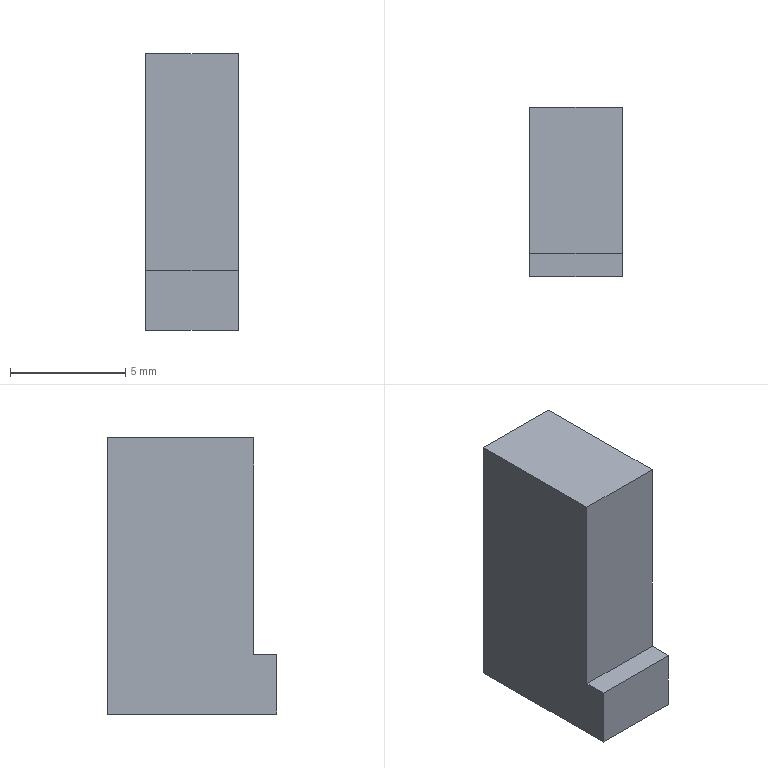Part | STEP file | lll_id462_x_t | 1 solid | 8 faces | box 4 x 7.35 x 12 mm | volume 315.2 mm3 | plane 8
STEP:
#1=CARTESIAN_POINT('',(275.5,-169.675,-9.4));
#2=VERTEX_POINT('',#1);
#3=CARTESIAN_POINT('',(275.5,-168.675,-9.4));
#4=VERTEX_POINT('',#3);
#5=CARTESIAN_POINT('',(275.5,-169.675,-9.4));
#6=DIRECTION('',(0.,1.,0.));
#7=VECTOR('',#6,1.);
#8=LINE('',#5,#7);
#9=EDGE_CURVE('',#2,#4,#8,.T.);
#10=ORIENTED_EDGE('',*,*,#9,.F.);
#11=CARTESIAN_POINT('',(279.5,-169.675,-9.4));
#12=VERTEX_POINT('',#11);
#13=CARTESIAN_POINT('',(279.5,-169.675,-9.4));
#14=DIRECTION('',(-1.,0.,0.));
#15=VECTOR('',#14,1.);
#16=LINE('',#13,#15);
#17=EDGE_CURVE('',#12,#2,#16,.T.);
#18=ORIENTED_EDGE('',*,*,#17,.F.);
#19=CARTESIAN_POINT('',(279.5,-168.675,-9.4));
#20=VERTEX_POINT('',#19);
#21=CARTESIAN_POINT('',(279.5,-169.675,-9.4));
#22=DIRECTION('',(0.,1.,0.));
#23=VECTOR('',#22,1.);
#24=LINE('',#21,#23);
#25=EDGE_CURVE('',#12,#20,#24,.T.);
#26=ORIENTED_EDGE('',*,*,#25,.T.);
#27=CARTESIAN_POINT('',(279.5,-168.675,-9.4));
#28=DIRECTION('',(-1.,0.,0.));
#29=VECTOR('',#28,1.);
#30=LINE('',#27,#29);
#31=EDGE_CURVE('',#20,#4,#30,.T.);
#32=ORIENTED_EDGE('',*,*,#31,.T.);
#33=EDGE_LOOP('',(#10,#18,#26,#32));
#34=FACE_OUTER_BOUND('',#33,.T.);
#35=CARTESIAN_POINT('',(279.5,-169.675,-9.4));
#36=DIRECTION('',(0.,0.,1.));
#37=DIRECTION('',(1.,0.,0.));
#38=AXIS2_PLACEMENT_3D('',#35,#36,#37);
#39=PLANE('',#38);
#40=ADVANCED_FACE('',(#34),#39,.T.);
#41=CARTESIAN_POINT('',(275.5,-168.675,0.));
#42=VERTEX_POINT('',#41);
#43=CARTESIAN_POINT('',(275.5,-168.675,0.));
#44=DIRECTION('',(0.,0.,-1.));
#45=VECTOR('',#44,1.);
#46=LINE('',#43,#45);
#47=EDGE_CURVE('',#42,#4,#46,.T.);
#48=ORIENTED_EDGE('',*,*,#47,.T.);
#49=ORIENTED_EDGE('',*,*,#31,.F.);
#50=CARTESIAN_POINT('',(279.5,-168.675,0.));
#51=VERTEX_POINT('',#50);
#52=CARTESIAN_POINT('',(279.5,-168.675,0.));
#53=DIRECTION('',(0.,0.,-1.));
#54=VECTOR('',#53,1.);
#55=LINE('',#52,#54);
#56=EDGE_CURVE('',#51,#20,#55,.T.);
#57=ORIENTED_EDGE('',*,*,#56,.F.);
#58=CARTESIAN_POINT('',(279.5,-168.675,0.));
#59=DIRECTION('',(-1.,0.,0.));
#60=VECTOR('',#59,1.);
#61=LINE('',#58,#60);
#62=EDGE_CURVE('',#51,#42,#61,.T.);
#63=ORIENTED_EDGE('',*,*,#62,.T.);
#64=EDGE_LOOP('',(#48,#49,#57,#63));
#65=FACE_OUTER_BOUND('',#64,.T.);
#66=CARTESIAN_POINT('',(279.5,-168.675,0.));
#67=DIRECTION('',(0.,1.,0.));
#68=DIRECTION('',(0.,0.,1.));
#69=AXIS2_PLACEMENT_3D('',#66,#67,#68);
#70=PLANE('',#69);
#71=ADVANCED_FACE('',(#65),#70,.F.);
#72=CARTESIAN_POINT('',(275.5,-162.325,0.));
#73=VERTEX_POINT('',#72);
#74=CARTESIAN_POINT('',(275.5,-162.325,0.));
#75=DIRECTION('',(0.,-1.,0.));
#76=VECTOR('',#75,1.);
#77=LINE('',#74,#76);
#78=EDGE_CURVE('',#73,#42,#77,.T.);
#79=ORIENTED_EDGE('',*,*,#78,.T.);
#80=ORIENTED_EDGE('',*,*,#62,.F.);
#81=CARTESIAN_POINT('',(279.5,-162.325,0.));
#82=VERTEX_POINT('',#81);
#83=CARTESIAN_POINT('',(279.5,-162.325,0.));
#84=DIRECTION('',(0.,-1.,0.));
#85=VECTOR('',#84,1.);
#86=LINE('',#83,#85);
#87=EDGE_CURVE('',#82,#51,#86,.T.);
#88=ORIENTED_EDGE('',*,*,#87,.F.);
#89=CARTESIAN_POINT('',(279.5,-162.325,0.));
#90=DIRECTION('',(-1.,0.,0.));
#91=VECTOR('',#90,1.);
#92=LINE('',#89,#91);
#93=EDGE_CURVE('',#82,#73,#92,.T.);
#94=ORIENTED_EDGE('',*,*,#93,.T.);
#95=EDGE_LOOP('',(#79,#80,#88,#94));
#96=FACE_OUTER_BOUND('',#95,.T.);
#97=CARTESIAN_POINT('',(279.5,-162.325,0.));
#98=DIRECTION('',(0.,0.,-1.));
#99=DIRECTION('',(-1.,0.,0.));
#100=AXIS2_PLACEMENT_3D('',#97,#98,#99);
#101=PLANE('',#100);
#102=ADVANCED_FACE('',(#96),#101,.F.);
#103=CARTESIAN_POINT('',(275.5,-162.325,-12.));
#104=VERTEX_POINT('',#103);
#105=CARTESIAN_POINT('',(275.5,-162.325,0.));
#106=DIRECTION('',(0.,0.,-1.));
#107=VECTOR('',#106,1.);
#108=LINE('',#105,#107);
#109=EDGE_CURVE('',#73,#104,#108,.T.);
#110=ORIENTED_EDGE('',*,*,#109,.F.);
#111=ORIENTED_EDGE('',*,*,#93,.F.);
#112=CARTESIAN_POINT('',(279.5,-162.325,-12.));
#113=VERTEX_POINT('',#112);
#114=CARTESIAN_POINT('',(279.5,-162.325,0.));
#115=DIRECTION('',(0.,0.,-1.));
#116=VECTOR('',#115,1.);
#117=LINE('',#114,#116);
#118=EDGE_CURVE('',#82,#113,#117,.T.);
#119=ORIENTED_EDGE('',*,*,#118,.T.);
#120=CARTESIAN_POINT('',(279.5,-162.325,-12.));
#121=DIRECTION('',(-1.,0.,0.));
#122=VECTOR('',#121,1.);
#123=LINE('',#120,#122);
#124=EDGE_CURVE('',#113,#104,#123,.T.);
#125=ORIENTED_EDGE('',*,*,#124,.T.);
#126=EDGE_LOOP('',(#110,#111,#119,#125));
#127=FACE_OUTER_BOUND('',#126,.T.);
#128=CARTESIAN_POINT('',(279.5,-162.325,0.));
#129=DIRECTION('',(0.,1.,0.));
#130=DIRECTION('',(0.,0.,1.));
#131=AXIS2_PLACEMENT_3D('',#128,#129,#130);
#132=PLANE('',#131);
#133=ADVANCED_FACE('',(#127),#132,.T.);
#134=CARTESIAN_POINT('',(275.5,-169.675,-12.));
#135=VERTEX_POINT('',#134);
#136=CARTESIAN_POINT('',(275.5,-169.675,-12.));
#137=DIRECTION('',(0.,1.,0.));
#138=VECTOR('',#137,1.);
#139=LINE('',#136,#138);
#140=EDGE_CURVE('',#135,#104,#139,.T.);
#141=ORIENTED_EDGE('',*,*,#140,.T.);
#142=ORIENTED_EDGE('',*,*,#124,.F.);
#143=CARTESIAN_POINT('',(279.5,-169.675,-12.));
#144=VERTEX_POINT('',#143);
#145=CARTESIAN_POINT('',(279.5,-169.675,-12.));
#146=DIRECTION('',(0.,1.,0.));
#147=VECTOR('',#146,1.);
#148=LINE('',#145,#147);
#149=EDGE_CURVE('',#144,#113,#148,.T.);
#150=ORIENTED_EDGE('',*,*,#149,.F.);
#151=CARTESIAN_POINT('',(279.5,-169.675,-12.));
#152=DIRECTION('',(-1.,0.,0.));
#153=VECTOR('',#152,1.);
#154=LINE('',#151,#153);
#155=EDGE_CURVE('',#144,#135,#154,.T.);
#156=ORIENTED_EDGE('',*,*,#155,.T.);
#157=EDGE_LOOP('',(#141,#142,#150,#156));
#158=FACE_OUTER_BOUND('',#157,.T.);
#159=CARTESIAN_POINT('',(279.5,-169.675,-12.));
#160=DIRECTION('',(0.,0.,1.));
#161=DIRECTION('',(1.,0.,0.));
#162=AXIS2_PLACEMENT_3D('',#159,#160,#161);
#163=PLANE('',#162);
#164=ADVANCED_FACE('',(#158),#163,.F.);
#165=CARTESIAN_POINT('',(275.5,-169.675,-9.4));
#166=DIRECTION('',(0.,0.,-1.));
#167=VECTOR('',#166,1.);
#168=LINE('',#165,#167);
#169=EDGE_CURVE('',#2,#135,#168,.T.);
#170=ORIENTED_EDGE('',*,*,#169,.T.);
#171=ORIENTED_EDGE('',*,*,#155,.F.);
#172=CARTESIAN_POINT('',(279.5,-169.675,-9.4));
#173=DIRECTION('',(0.,0.,-1.));
#174=VECTOR('',#173,1.);
#175=LINE('',#172,#174);
#176=EDGE_CURVE('',#12,#144,#175,.T.);
#177=ORIENTED_EDGE('',*,*,#176,.F.);
#178=ORIENTED_EDGE('',*,*,#17,.T.);
#179=EDGE_LOOP('',(#170,#171,#177,#178));
#180=FACE_OUTER_BOUND('',#179,.T.);
#181=CARTESIAN_POINT('',(279.5,-169.675,-9.4));
#182=DIRECTION('',(0.,1.,0.));
#183=DIRECTION('',(0.,0.,1.));
#184=AXIS2_PLACEMENT_3D('',#181,#182,#183);
#185=PLANE('',#184);
#186=ADVANCED_FACE('',(#180),#185,.F.);
#187=ORIENTED_EDGE('',*,*,#25,.F.);
#188=ORIENTED_EDGE('',*,*,#176,.T.);
#189=ORIENTED_EDGE('',*,*,#149,.T.);
#190=ORIENTED_EDGE('',*,*,#118,.F.);
#191=ORIENTED_EDGE('',*,*,#87,.T.);
#192=ORIENTED_EDGE('',*,*,#56,.T.);
#193=EDGE_LOOP('',(#187,#188,#189,#190,#191,#192));
#194=FACE_OUTER_BOUND('',#193,.T.);
#195=CARTESIAN_POINT('',(279.5,0.,0.));
#196=DIRECTION('',(-1.,0.,0.));
#197=DIRECTION('',(0.,0.,1.));
#198=AXIS2_PLACEMENT_3D('',#195,#196,#197);
#199=PLANE('',#198);
#200=ADVANCED_FACE('',(#194),#199,.F.);
#201=ORIENTED_EDGE('',*,*,#9,.T.);
#202=ORIENTED_EDGE('',*,*,#47,.F.);
#203=ORIENTED_EDGE('',*,*,#78,.F.);
#204=ORIENTED_EDGE('',*,*,#109,.T.);
#205=ORIENTED_EDGE('',*,*,#140,.F.);
#206=ORIENTED_EDGE('',*,*,#169,.F.);
#207=EDGE_LOOP('',(#201,#202,#203,#204,#205,#206));
#208=FACE_OUTER_BOUND('',#207,.T.);
#209=CARTESIAN_POINT('',(275.5,0.,0.));
#210=DIRECTION('',(-1.,0.,0.));
#211=DIRECTION('',(0.,0.,1.));
#212=AXIS2_PLACEMENT_3D('',#209,#210,#211);
#213=PLANE('',#212);
#214=ADVANCED_FACE('',(#208),#213,.T.);
#215=CLOSED_SHELL('',(#40,#71,#102,#133,#164,#186,#200,#214));
#216=MANIFOLD_SOLID_BREP('',#215);
#217=(LENGTH_UNIT()NAMED_UNIT(*)SI_UNIT(.MILLI.,.METRE.));
#218=UNCERTAINTY_MEASURE_WITH_UNIT(LENGTH_MEASURE(0.00002),#217,'','');
#219=(NAMED_UNIT(*)PLANE_ANGLE_UNIT()SI_UNIT($,.RADIAN.));
#220=PLANE_ANGLE_MEASURE_WITH_UNIT(PLANE_ANGLE_MEASURE(0.01745),#219);
#221=DIMENSIONAL_EXPONENTS(0.,0.,0.,0.,0.,0.,0.);
#222=(CONVERSION_BASED_UNIT('DEGREE',#220)NAMED_UNIT(#221)PLANE_ANGLE_UNIT());
#223=(NAMED_UNIT(*)SI_UNIT($,.STERADIAN.)SOLID_ANGLE_UNIT());
#224=(GEOMETRIC_REPRESENTATION_CONTEXT(3)GLOBAL_UNCERTAINTY_ASSIGNED_CONTEXT((#218))GLOBAL_UNIT_ASSIGNED_CONTEXT((#217,#222,#223))REPRESENTATION_CONTEXT('',''));
#225=ADVANCED_BREP_SHAPE_REPRESENTATION('',(#216),#224);